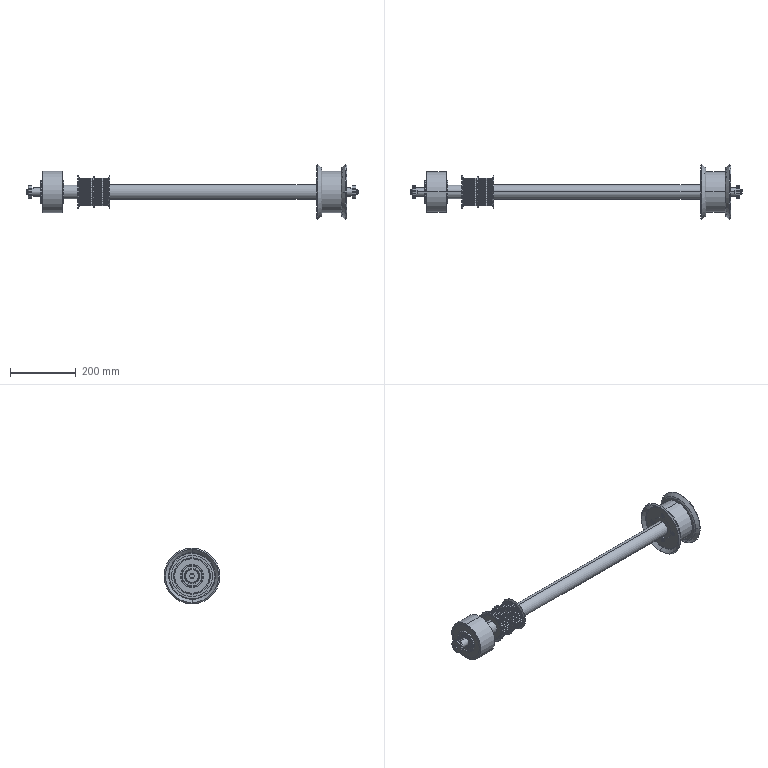Part | SolidWorks | 35 solids | 1802 faces | box 1011 x 169.042 x 169.042 mm | volume 2962716 mm3 | cylinder 844 | plane 498 | cone 288 | spline 172 | commonest cylinder face diameters 6 x200 1.6 x168 5.14 x168 85.208 x70 5 x16 6.6 x16